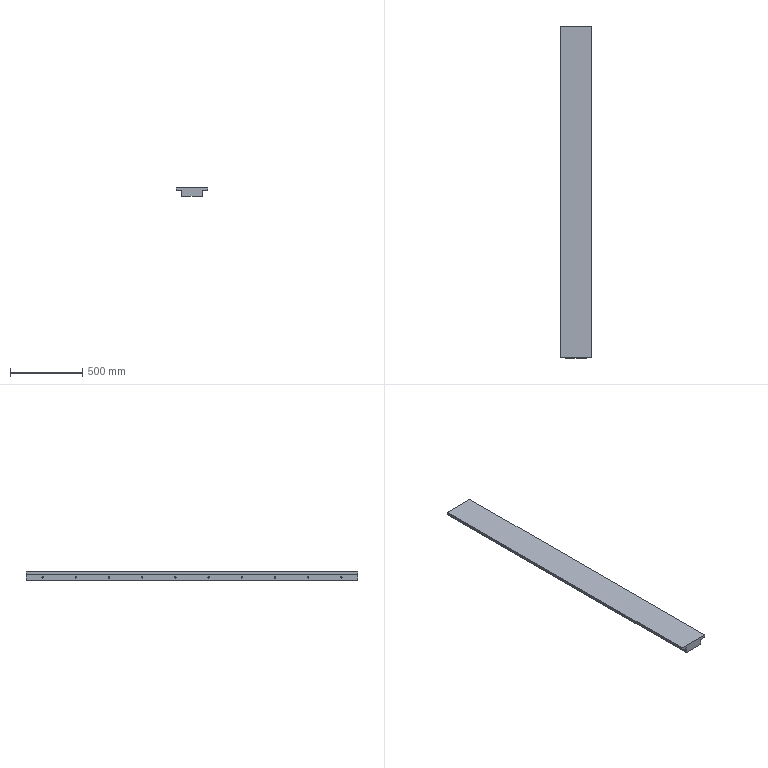Part | SolidWorks | features Extrusion 1, HoleWzd 1, LPattern 1, MirrorPattern 1 | 1 solid | 130 faces | box 220 x 2300 x 60 mm | volume 22970661 mm3 | cone 80 | cylinder 40 | plane 10 | commonest cylinder face diameters 8.5 x40